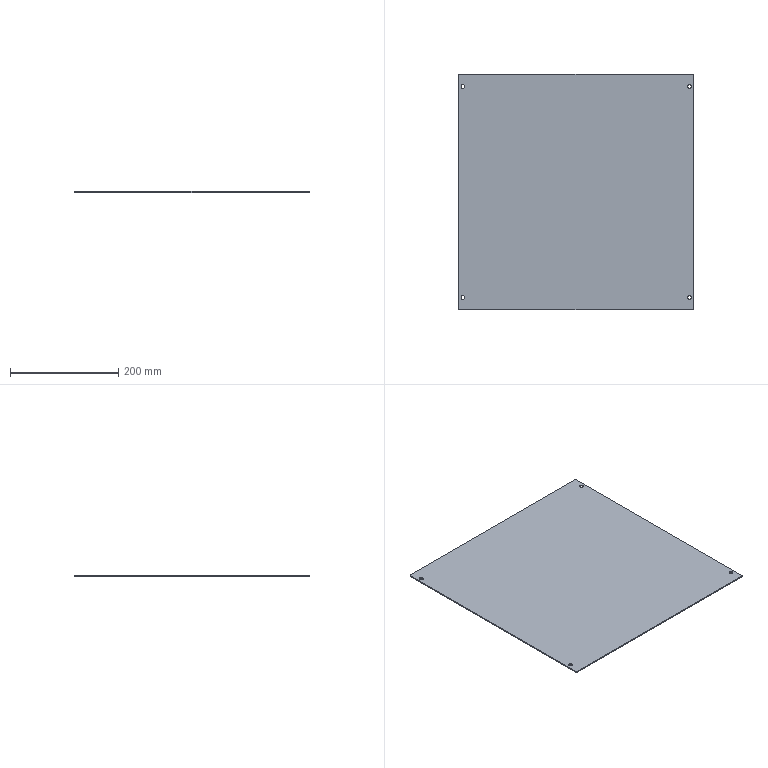Part | STEP file | Control Box Rear Closing Plate | 1 solid | 18 faces | box 433 x 435 x 2 mm | volume 376395 mm3 | cylinder 12 | plane 6 | commonest cylinder face diameters 7 x8 4 x4
STEP:
#1=CARTESIAN_POINT('',(-411.682,-25.867,-2.));
#2=VERTEX_POINT('',#1);
#3=CARTESIAN_POINT('',(-418.682,-25.867,-2.));
#4=VERTEX_POINT('',#3);
#5=CARTESIAN_POINT('',(-415.182,-25.867,-2.));
#6=DIRECTION('',(0.,0.,-1.));
#7=DIRECTION('',(1.,0.,0.));
#8=AXIS2_PLACEMENT_3D('',#5,#6,#7);
#9=CIRCLE('',#8,3.5);
#10=EDGE_CURVE('',#2,#4,#9,.T.);
#11=ORIENTED_EDGE('',*,*,#10,.T.);
#12=CARTESIAN_POINT('',(-418.682,-25.867,0.));
#13=VERTEX_POINT('',#12);
#14=CARTESIAN_POINT('',(-418.682,-25.867,-10.));
#15=DIRECTION('',(0.,0.,1.));
#16=VECTOR('',#15,1000.);
#17=LINE('',#14,#16);
#18=EDGE_CURVE('',#4,#13,#17,.T.);
#19=ORIENTED_EDGE('',*,*,#18,.T.);
#20=CARTESIAN_POINT('',(-411.682,-25.867,0.));
#21=VERTEX_POINT('',#20);
#22=CARTESIAN_POINT('',(-415.182,-25.867,0.));
#23=DIRECTION('',(0.,0.,-1.));
#24=DIRECTION('',(1.,0.,0.));
#25=AXIS2_PLACEMENT_3D('',#22,#23,#24);
#26=CIRCLE('',#25,3.5);
#27=EDGE_CURVE('',#21,#13,#26,.T.);
#28=ORIENTED_EDGE('',*,*,#27,.F.);
#29=CARTESIAN_POINT('',(-411.682,-25.867,-10.));
#30=DIRECTION('',(0.,0.,1.));
#31=VECTOR('',#30,1000.);
#32=LINE('',#29,#31);
#33=EDGE_CURVE('',#2,#21,#32,.T.);
#34=ORIENTED_EDGE('',*,*,#33,.F.);
#35=EDGE_LOOP('',(#11,#19,#28,#34));
#36=FACE_OUTER_BOUND('',#35,.T.);
#37=CARTESIAN_POINT('',(-415.182,-25.867,-10.));
#38=DIRECTION('',(0.,0.,1.));
#39=DIRECTION('',(1.,0.,0.));
#40=AXIS2_PLACEMENT_3D('',#37,#38,#39);
#41=CYLINDRICAL_SURFACE('',#40,3.5);
#42=ADVANCED_FACE('',(#36),#41,.F.);
#43=CARTESIAN_POINT('',(6.197,-25.867,-2.));
#44=VERTEX_POINT('',#43);
#45=CARTESIAN_POINT('',(-0.8031,-25.867,-2.));
#46=VERTEX_POINT('',#45);
#47=CARTESIAN_POINT('',(2.697,-25.867,-2.));
#48=DIRECTION('',(0.,0.,-1.));
#49=DIRECTION('',(1.,0.,0.));
#50=AXIS2_PLACEMENT_3D('',#47,#48,#49);
#51=CIRCLE('',#50,3.5);
#52=EDGE_CURVE('',#44,#46,#51,.T.);
#53=ORIENTED_EDGE('',*,*,#52,.T.);
#54=CARTESIAN_POINT('',(-0.8031,-25.867,0.));
#55=VERTEX_POINT('',#54);
#56=CARTESIAN_POINT('',(-0.8031,-25.867,-10.));
#57=DIRECTION('',(0.,0.,1.));
#58=VECTOR('',#57,1000.);
#59=LINE('',#56,#58);
#60=EDGE_CURVE('',#46,#55,#59,.T.);
#61=ORIENTED_EDGE('',*,*,#60,.T.);
#62=CARTESIAN_POINT('',(6.197,-25.867,0.));
#63=VERTEX_POINT('',#62);
#64=CARTESIAN_POINT('',(2.697,-25.867,0.));
#65=DIRECTION('',(0.,0.,-1.));
#66=DIRECTION('',(1.,0.,0.));
#67=AXIS2_PLACEMENT_3D('',#64,#65,#66);
#68=CIRCLE('',#67,3.5);
#69=EDGE_CURVE('',#63,#55,#68,.T.);
#70=ORIENTED_EDGE('',*,*,#69,.F.);
#71=CARTESIAN_POINT('',(6.197,-25.867,-10.));
#72=DIRECTION('',(0.,0.,1.));
#73=VECTOR('',#72,1000.);
#74=LINE('',#71,#73);
#75=EDGE_CURVE('',#44,#63,#74,.T.);
#76=ORIENTED_EDGE('',*,*,#75,.F.);
#77=EDGE_LOOP('',(#53,#61,#70,#76));
#78=FACE_OUTER_BOUND('',#77,.T.);
#79=CARTESIAN_POINT('',(2.697,-25.867,-10.));
#80=DIRECTION('',(0.,0.,1.));
#81=DIRECTION('',(1.,0.,0.));
#82=AXIS2_PLACEMENT_3D('',#79,#80,#81);
#83=CYLINDRICAL_SURFACE('',#82,3.5);
#84=ADVANCED_FACE('',(#78),#83,.F.);
#85=CARTESIAN_POINT('',(6.197,-414.867,-2.));
#86=VERTEX_POINT('',#85);
#87=CARTESIAN_POINT('',(-0.8031,-414.867,-2.));
#88=VERTEX_POINT('',#87);
#89=CARTESIAN_POINT('',(2.697,-414.867,-2.));
#90=DIRECTION('',(0.,0.,-1.));
#91=DIRECTION('',(1.,0.,0.));
#92=AXIS2_PLACEMENT_3D('',#89,#90,#91);
#93=CIRCLE('',#92,3.5);
#94=EDGE_CURVE('',#86,#88,#93,.T.);
#95=ORIENTED_EDGE('',*,*,#94,.T.);
#96=CARTESIAN_POINT('',(-0.8031,-414.867,0.));
#97=VERTEX_POINT('',#96);
#98=CARTESIAN_POINT('',(-0.8031,-414.867,-10.));
#99=DIRECTION('',(0.,0.,1.));
#100=VECTOR('',#99,1000.);
#101=LINE('',#98,#100);
#102=EDGE_CURVE('',#88,#97,#101,.T.);
#103=ORIENTED_EDGE('',*,*,#102,.T.);
#104=CARTESIAN_POINT('',(6.197,-414.867,0.));
#105=VERTEX_POINT('',#104);
#106=CARTESIAN_POINT('',(2.697,-414.867,0.));
#107=DIRECTION('',(0.,0.,-1.));
#108=DIRECTION('',(1.,0.,0.));
#109=AXIS2_PLACEMENT_3D('',#106,#107,#108);
#110=CIRCLE('',#109,3.5);
#111=EDGE_CURVE('',#105,#97,#110,.T.);
#112=ORIENTED_EDGE('',*,*,#111,.F.);
#113=CARTESIAN_POINT('',(6.197,-414.867,-10.));
#114=DIRECTION('',(0.,0.,1.));
#115=VECTOR('',#114,1000.);
#116=LINE('',#113,#115);
#117=EDGE_CURVE('',#86,#105,#116,.T.);
#118=ORIENTED_EDGE('',*,*,#117,.F.);
#119=EDGE_LOOP('',(#95,#103,#112,#118));
#120=FACE_OUTER_BOUND('',#119,.T.);
#121=CARTESIAN_POINT('',(2.697,-414.867,-10.));
#122=DIRECTION('',(0.,0.,1.));
#123=DIRECTION('',(1.,0.,0.));
#124=AXIS2_PLACEMENT_3D('',#121,#122,#123);
#125=CYLINDRICAL_SURFACE('',#124,3.5);
#126=ADVANCED_FACE('',(#120),#125,.F.);
#127=CARTESIAN_POINT('',(-411.682,-414.867,-2.));
#128=VERTEX_POINT('',#127);
#129=CARTESIAN_POINT('',(-418.682,-414.867,-2.));
#130=VERTEX_POINT('',#129);
#131=CARTESIAN_POINT('',(-415.182,-414.867,-2.));
#132=DIRECTION('',(0.,0.,-1.));
#133=DIRECTION('',(1.,0.,0.));
#134=AXIS2_PLACEMENT_3D('',#131,#132,#133);
#135=CIRCLE('',#134,3.5);
#136=EDGE_CURVE('',#128,#130,#135,.T.);
#137=ORIENTED_EDGE('',*,*,#136,.T.);
#138=CARTESIAN_POINT('',(-418.682,-414.867,0.));
#139=VERTEX_POINT('',#138);
#140=CARTESIAN_POINT('',(-418.682,-414.867,-10.));
#141=DIRECTION('',(0.,0.,1.));
#142=VECTOR('',#141,1000.);
#143=LINE('',#140,#142);
#144=EDGE_CURVE('',#130,#139,#143,.T.);
#145=ORIENTED_EDGE('',*,*,#144,.T.);
#146=CARTESIAN_POINT('',(-411.682,-414.867,0.));
#147=VERTEX_POINT('',#146);
#148=CARTESIAN_POINT('',(-415.182,-414.867,0.));
#149=DIRECTION('',(0.,0.,-1.));
#150=DIRECTION('',(1.,0.,0.));
#151=AXIS2_PLACEMENT_3D('',#148,#149,#150);
#152=CIRCLE('',#151,3.5);
#153=EDGE_CURVE('',#147,#139,#152,.T.);
#154=ORIENTED_EDGE('',*,*,#153,.F.);
#155=CARTESIAN_POINT('',(-411.682,-414.867,-10.));
#156=DIRECTION('',(0.,0.,1.));
#157=VECTOR('',#156,1000.);
#158=LINE('',#155,#157);
#159=EDGE_CURVE('',#128,#147,#158,.T.);
#160=ORIENTED_EDGE('',*,*,#159,.F.);
#161=EDGE_LOOP('',(#137,#145,#154,#160));
#162=FACE_OUTER_BOUND('',#161,.T.);
#163=CARTESIAN_POINT('',(-415.182,-414.867,-10.));
#164=DIRECTION('',(0.,0.,1.));
#165=DIRECTION('',(1.,0.,0.));
#166=AXIS2_PLACEMENT_3D('',#163,#164,#165);
#167=CYLINDRICAL_SURFACE('',#166,3.5);
#168=ADVANCED_FACE('',(#162),#167,.F.);
#169=CARTESIAN_POINT('',(7.818,-437.867,-2.));
#170=VERTEX_POINT('',#169);
#171=CARTESIAN_POINT('',(9.818,-435.867,-2.));
#172=VERTEX_POINT('',#171);
#173=CARTESIAN_POINT('',(7.818,-435.867,-2.));
#174=DIRECTION('',(0.,0.,1.));
#175=DIRECTION('',(1.,0.,0.));
#176=AXIS2_PLACEMENT_3D('',#173,#174,#175);
#177=CIRCLE('',#176,2.);
#178=EDGE_CURVE('',#170,#172,#177,.T.);
#179=ORIENTED_EDGE('',*,*,#178,.F.);
#180=CARTESIAN_POINT('',(-421.182,-437.867,-2.));
#181=VERTEX_POINT('',#180);
#182=CARTESIAN_POINT('',(0.,-437.867,-2.));
#183=DIRECTION('',(1.,0.,0.));
#184=VECTOR('',#183,1000.);
#185=LINE('',#182,#184);
#186=EDGE_CURVE('',#181,#170,#185,.T.);
#187=ORIENTED_EDGE('',*,*,#186,.F.);
#188=CARTESIAN_POINT('',(-423.182,-435.867,-2.));
#189=VERTEX_POINT('',#188);
#190=CARTESIAN_POINT('',(-421.182,-435.867,-2.));
#191=DIRECTION('',(0.,0.,1.));
#192=DIRECTION('',(1.,0.,0.));
#193=AXIS2_PLACEMENT_3D('',#190,#191,#192);
#194=CIRCLE('',#193,2.);
#195=EDGE_CURVE('',#189,#181,#194,.T.);
#196=ORIENTED_EDGE('',*,*,#195,.F.);
#197=CARTESIAN_POINT('',(-423.182,-4.867,-2.));
#198=VERTEX_POINT('',#197);
#199=CARTESIAN_POINT('',(-423.182,0.,-2.));
#200=DIRECTION('',(0.,-1.,0.));
#201=VECTOR('',#200,1000.);
#202=LINE('',#199,#201);
#203=EDGE_CURVE('',#198,#189,#202,.T.);
#204=ORIENTED_EDGE('',*,*,#203,.F.);
#205=CARTESIAN_POINT('',(-421.182,-2.867,-2.));
#206=VERTEX_POINT('',#205);
#207=CARTESIAN_POINT('',(-421.182,-4.867,-2.));
#208=DIRECTION('',(0.,0.,1.));
#209=DIRECTION('',(1.,0.,0.));
#210=AXIS2_PLACEMENT_3D('',#207,#208,#209);
#211=CIRCLE('',#210,2.);
#212=EDGE_CURVE('',#206,#198,#211,.T.);
#213=ORIENTED_EDGE('',*,*,#212,.F.);
#214=CARTESIAN_POINT('',(7.818,-2.867,-2.));
#215=VERTEX_POINT('',#214);
#216=CARTESIAN_POINT('',(0.,-2.867,-2.));
#217=DIRECTION('',(-1.,0.,0.));
#218=VECTOR('',#217,1000.);
#219=LINE('',#216,#218);
#220=EDGE_CURVE('',#215,#206,#219,.T.);
#221=ORIENTED_EDGE('',*,*,#220,.F.);
#222=CARTESIAN_POINT('',(9.818,-4.867,-2.));
#223=VERTEX_POINT('',#222);
#224=CARTESIAN_POINT('',(7.818,-4.867,-2.));
#225=DIRECTION('',(0.,0.,1.));
#226=DIRECTION('',(1.,0.,0.));
#227=AXIS2_PLACEMENT_3D('',#224,#225,#226);
#228=CIRCLE('',#227,2.);
#229=EDGE_CURVE('',#223,#215,#228,.T.);
#230=ORIENTED_EDGE('',*,*,#229,.F.);
#231=CARTESIAN_POINT('',(9.818,0.,-2.));
#232=DIRECTION('',(0.,1.,0.));
#233=VECTOR('',#232,1000.);
#234=LINE('',#231,#233);
#235=EDGE_CURVE('',#172,#223,#234,.T.);
#236=ORIENTED_EDGE('',*,*,#235,.F.);
#237=EDGE_LOOP('',(#179,#187,#196,#204,#213,#221,#230,#236));
#238=FACE_OUTER_BOUND('',#237,.T.);
#239=ORIENTED_EDGE('',*,*,#10,.F.);
#240=CARTESIAN_POINT('',(-415.182,-25.867,-2.));
#241=DIRECTION('',(0.,0.,-1.));
#242=DIRECTION('',(1.,0.,0.));
#243=AXIS2_PLACEMENT_3D('',#240,#241,#242);
#244=CIRCLE('',#243,3.5);
#245=EDGE_CURVE('',#4,#2,#244,.T.);
#246=ORIENTED_EDGE('',*,*,#245,.F.);
#247=EDGE_LOOP('',(#239,#246));
#248=FACE_BOUND('',#247,.T.);
#249=ORIENTED_EDGE('',*,*,#52,.F.);
#250=CARTESIAN_POINT('',(2.697,-25.867,-2.));
#251=DIRECTION('',(0.,0.,-1.));
#252=DIRECTION('',(1.,0.,0.));
#253=AXIS2_PLACEMENT_3D('',#250,#251,#252);
#254=CIRCLE('',#253,3.5);
#255=EDGE_CURVE('',#46,#44,#254,.T.);
#256=ORIENTED_EDGE('',*,*,#255,.F.);
#257=EDGE_LOOP('',(#249,#256));
#258=FACE_BOUND('',#257,.T.);
#259=ORIENTED_EDGE('',*,*,#94,.F.);
#260=CARTESIAN_POINT('',(2.697,-414.867,-2.));
#261=DIRECTION('',(0.,0.,-1.));
#262=DIRECTION('',(1.,0.,0.));
#263=AXIS2_PLACEMENT_3D('',#260,#261,#262);
#264=CIRCLE('',#263,3.5);
#265=EDGE_CURVE('',#88,#86,#264,.T.);
#266=ORIENTED_EDGE('',*,*,#265,.F.);
#267=EDGE_LOOP('',(#259,#266));
#268=FACE_BOUND('',#267,.T.);
#269=ORIENTED_EDGE('',*,*,#136,.F.);
#270=CARTESIAN_POINT('',(-415.182,-414.867,-2.));
#271=DIRECTION('',(0.,0.,-1.));
#272=DIRECTION('',(1.,0.,0.));
#273=AXIS2_PLACEMENT_3D('',#270,#271,#272);
#274=CIRCLE('',#273,3.5);
#275=EDGE_CURVE('',#130,#128,#274,.T.);
#276=ORIENTED_EDGE('',*,*,#275,.F.);
#277=EDGE_LOOP('',(#269,#276));
#278=FACE_BOUND('',#277,.T.);
#279=CARTESIAN_POINT('',(0.,0.,-2.));
#280=DIRECTION('',(0.,0.,1.));
#281=DIRECTION('',(1.,0.,0.));
#282=AXIS2_PLACEMENT_3D('',#279,#280,#281);
#283=PLANE('',#282);
#284=ADVANCED_FACE('',(#238,#248,#258,#268,#278),#283,.F.);
#285=ORIENTED_EDGE('',*,*,#235,.T.);
#286=CARTESIAN_POINT('',(9.818,-4.867,0.));
#287=VERTEX_POINT('',#286);
#288=CARTESIAN_POINT('',(9.818,-4.867,-2.));
#289=DIRECTION('',(0.,0.,1.));
#290=VECTOR('',#289,1000.);
#291=LINE('',#288,#290);
#292=EDGE_CURVE('',#223,#287,#291,.T.);
#293=ORIENTED_EDGE('',*,*,#292,.T.);
#294=CARTESIAN_POINT('',(9.818,-435.867,0.));
#295=VERTEX_POINT('',#294);
#296=CARTESIAN_POINT('',(9.818,-2.867,0.));
#297=DIRECTION('',(0.,-1.,0.));
#298=VECTOR('',#297,1000.);
#299=LINE('',#296,#298);
#300=EDGE_CURVE('',#287,#295,#299,.T.);
#301=ORIENTED_EDGE('',*,*,#300,.T.);
#302=CARTESIAN_POINT('',(9.818,-435.867,-2.));
#303=DIRECTION('',(0.,0.,-1.));
#304=VECTOR('',#303,1000.);
#305=LINE('',#302,#304);
#306=EDGE_CURVE('',#295,#172,#305,.T.);
#307=ORIENTED_EDGE('',*,*,#306,.T.);
#308=EDGE_LOOP('',(#285,#293,#301,#307));
#309=FACE_OUTER_BOUND('',#308,.T.);
#310=CARTESIAN_POINT('',(9.818,-2.867,-2.));
#311=DIRECTION('',(1.,0.,0.));
#312=DIRECTION('',(0.,1.,0.));
#313=AXIS2_PLACEMENT_3D('',#310,#311,#312);
#314=PLANE('',#313);
#315=ADVANCED_FACE('',(#309),#314,.T.);
#316=CARTESIAN_POINT('',(7.818,-437.867,0.));
#317=VERTEX_POINT('',#316);
#318=CARTESIAN_POINT('',(7.818,-435.867,0.));
#319=DIRECTION('',(0.,0.,-1.));
#320=DIRECTION('',(1.,0.,0.));
#321=AXIS2_PLACEMENT_3D('',#318,#319,#320);
#322=CIRCLE('',#321,2.);
#323=EDGE_CURVE('',#295,#317,#322,.T.);
#324=ORIENTED_EDGE('',*,*,#323,.T.);
#325=CARTESIAN_POINT('',(7.818,-437.867,-2.));
#326=DIRECTION('',(0.,0.,-1.));
#327=VECTOR('',#326,1000.);
#328=LINE('',#325,#327);
#329=EDGE_CURVE('',#317,#170,#328,.T.);
#330=ORIENTED_EDGE('',*,*,#329,.T.);
#331=ORIENTED_EDGE('',*,*,#178,.T.);
#332=ORIENTED_EDGE('',*,*,#306,.F.);
#333=EDGE_LOOP('',(#324,#330,#331,#332));
#334=FACE_OUTER_BOUND('',#333,.T.);
#335=CARTESIAN_POINT('',(7.818,-435.867,-2.));
#336=DIRECTION('',(0.,0.,1.));
#337=DIRECTION('',(1.,0.,0.));
#338=AXIS2_PLACEMENT_3D('',#335,#336,#337);
#339=CYLINDRICAL_SURFACE('',#338,2.);
#340=ADVANCED_FACE('',(#334),#339,.T.);
#341=CARTESIAN_POINT('',(-421.182,-437.867,0.));
#342=VERTEX_POINT('',#341);
#343=CARTESIAN_POINT('',(-423.182,-437.867,0.));
#344=DIRECTION('',(-1.,0.,0.));
#345=VECTOR('',#344,1000.);
#346=LINE('',#343,#345);
#347=EDGE_CURVE('',#317,#342,#346,.T.);
#348=ORIENTED_EDGE('',*,*,#347,.T.);
#349=CARTESIAN_POINT('',(-421.182,-437.867,-2.));
#350=DIRECTION('',(0.,0.,-1.));
#351=VECTOR('',#350,1000.);
#352=LINE('',#349,#351);
#353=EDGE_CURVE('',#342,#181,#352,.T.);
#354=ORIENTED_EDGE('',*,*,#353,.T.);
#355=ORIENTED_EDGE('',*,*,#186,.T.);
#356=ORIENTED_EDGE('',*,*,#329,.F.);
#357=EDGE_LOOP('',(#348,#354,#355,#356));
#358=FACE_OUTER_BOUND('',#357,.T.);
#359=CARTESIAN_POINT('',(-423.182,-437.867,-2.));
#360=DIRECTION('',(0.,-1.,0.));
#361=DIRECTION('',(0.,0.,-1.));
#362=AXIS2_PLACEMENT_3D('',#359,#360,#361);
#363=PLANE('',#362);
#364=ADVANCED_FACE('',(#358),#363,.T.);
#365=CARTESIAN_POINT('',(-423.182,-435.867,0.));
#366=VERTEX_POINT('',#365);
#367=CARTESIAN_POINT('',(-421.182,-435.867,0.));
#368=DIRECTION('',(0.,0.,-1.));
#369=DIRECTION('',(1.,0.,0.));
#370=AXIS2_PLACEMENT_3D('',#367,#368,#369);
#371=CIRCLE('',#370,2.);
#372=EDGE_CURVE('',#342,#366,#371,.T.);
#373=ORIENTED_EDGE('',*,*,#372,.T.);
#374=CARTESIAN_POINT('',(-423.182,-435.867,-2.));
#375=DIRECTION('',(0.,0.,-1.));
#376=VECTOR('',#375,1000.);
#377=LINE('',#374,#376);
#378=EDGE_CURVE('',#366,#189,#377,.T.);
#379=ORIENTED_EDGE('',*,*,#378,.T.);
#380=ORIENTED_EDGE('',*,*,#195,.T.);
#381=ORIENTED_EDGE('',*,*,#353,.F.);
#382=EDGE_LOOP('',(#373,#379,#380,#381));
#383=FACE_OUTER_BOUND('',#382,.T.);
#384=CARTESIAN_POINT('',(-421.182,-435.867,-2.));
#385=DIRECTION('',(0.,0.,1.));
#386=DIRECTION('',(1.,0.,0.));
#387=AXIS2_PLACEMENT_3D('',#384,#385,#386);
#388=CYLINDRICAL_SURFACE('',#387,2.);
#389=ADVANCED_FACE('',(#383),#388,.T.);
#390=CARTESIAN_POINT('',(-423.182,-4.867,0.));
#391=VERTEX_POINT('',#390);
#392=CARTESIAN_POINT('',(-423.182,-2.867,0.));
#393=DIRECTION('',(0.,1.,0.));
#394=VECTOR('',#393,1000.);
#395=LINE('',#392,#394);
#396=EDGE_CURVE('',#366,#391,#395,.T.);
#397=ORIENTED_EDGE('',*,*,#396,.T.);
#398=CARTESIAN_POINT('',(-423.182,-4.867,-2.));
#399=DIRECTION('',(0.,0.,-1.));
#400=VECTOR('',#399,1000.);
#401=LINE('',#398,#400);
#402=EDGE_CURVE('',#391,#198,#401,.T.);
#403=ORIENTED_EDGE('',*,*,#402,.T.);
#404=ORIENTED_EDGE('',*,*,#203,.T.);
#405=ORIENTED_EDGE('',*,*,#378,.F.);
#406=EDGE_LOOP('',(#397,#403,#404,#405));
#407=FACE_OUTER_BOUND('',#406,.T.);
#408=CARTESIAN_POINT('',(-423.182,-2.867,-2.));
#409=DIRECTION('',(-1.,0.,0.));
#410=DIRECTION('',(0.,0.,1.));
#411=AXIS2_PLACEMENT_3D('',#408,#409,#410);
#412=PLANE('',#411);
#413=ADVANCED_FACE('',(#407),#412,.T.);
#414=CARTESIAN_POINT('',(-421.182,-2.867,0.));
#415=VERTEX_POINT('',#414);
#416=CARTESIAN_POINT('',(-421.182,-4.867,0.));
#417=DIRECTION('',(0.,0.,-1.));
#418=DIRECTION('',(1.,0.,0.));
#419=AXIS2_PLACEMENT_3D('',#416,#417,#418);
#420=CIRCLE('',#419,2.);
#421=EDGE_CURVE('',#391,#415,#420,.T.);
#422=ORIENTED_EDGE('',*,*,#421,.T.);
#423=CARTESIAN_POINT('',(-421.182,-2.867,-2.));
#424=DIRECTION('',(0.,0.,-1.));
#425=VECTOR('',#424,1000.);
#426=LINE('',#423,#425);
#427=EDGE_CURVE('',#415,#206,#426,.T.);
#428=ORIENTED_EDGE('',*,*,#427,.T.);
#429=ORIENTED_EDGE('',*,*,#212,.T.);
#430=ORIENTED_EDGE('',*,*,#402,.F.);
#431=EDGE_LOOP('',(#422,#428,#429,#430));
#432=FACE_OUTER_BOUND('',#431,.T.);
#433=CARTESIAN_POINT('',(-421.182,-4.867,-2.));
#434=DIRECTION('',(0.,0.,1.));
#435=DIRECTION('',(1.,0.,0.));
#436=AXIS2_PLACEMENT_3D('',#433,#434,#435);
#437=CYLINDRICAL_SURFACE('',#436,2.);
#438=ADVANCED_FACE('',(#432),#437,.T.);
#439=CARTESIAN_POINT('',(7.818,-2.867,0.));
#440=VERTEX_POINT('',#439);
#441=CARTESIAN_POINT('',(-423.182,-2.867,0.));
#442=DIRECTION('',(1.,0.,0.));
#443=VECTOR('',#442,1000.);
#444=LINE('',#441,#443);
#445=EDGE_CURVE('',#415,#440,#444,.T.);
#446=ORIENTED_EDGE('',*,*,#445,.T.);
#447=CARTESIAN_POINT('',(7.818,-2.867,-2.));
#448=DIRECTION('',(0.,0.,-1.));
#449=VECTOR('',#448,1000.);
#450=LINE('',#447,#449);
#451=EDGE_CURVE('',#440,#215,#450,.T.);
#452=ORIENTED_EDGE('',*,*,#451,.T.);
#453=ORIENTED_EDGE('',*,*,#220,.T.);
#454=ORIENTED_EDGE('',*,*,#427,.F.);
#455=EDGE_LOOP('',(#446,#452,#453,#454));
#456=FACE_OUTER_BOUND('',#455,.T.);
#457=CARTESIAN_POINT('',(-423.182,-2.867,-2.));
#458=DIRECTION('',(0.,1.,0.));
#459=DIRECTION('',(0.,0.,1.));
#460=AXIS2_PLACEMENT_3D('',#457,#458,#459);
#461=PLANE('',#460);
#462=ADVANCED_FACE('',(#456),#461,.T.);
#463=CARTESIAN_POINT('',(7.818,-4.867,0.));
#464=DIRECTION('',(0.,0.,-1.));
#465=DIRECTION('',(1.,0.,0.));
#466=AXIS2_PLACEMENT_3D('',#463,#464,#465);
#467=CIRCLE('',#466,2.);
#468=EDGE_CURVE('',#440,#287,#467,.T.);
#469=ORIENTED_EDGE('',*,*,#468,.T.);
#470=ORIENTED_EDGE('',*,*,#292,.F.);
#471=ORIENTED_EDGE('',*,*,#229,.T.);
#472=ORIENTED_EDGE('',*,*,#451,.F.);
#473=EDGE_LOOP('',(#469,#470,#471,#472));
#474=FACE_OUTER_BOUND('',#473,.T.);
#475=CARTESIAN_POINT('',(7.818,-4.867,-2.));
#476=DIRECTION('',(0.,0.,1.));
#477=DIRECTION('',(1.,0.,0.));
#478=AXIS2_PLACEMENT_3D('',#475,#476,#477);
#479=CYLINDRICAL_SURFACE('',#478,2.);
#480=ADVANCED_FACE('',(#474),#479,.T.);
#481=ORIENTED_EDGE('',*,*,#18,.F.);
#482=ORIENTED_EDGE('',*,*,#245,.T.);
#483=ORIENTED_EDGE('',*,*,#33,.T.);
#484=CARTESIAN_POINT('',(-415.182,-25.867,0.));
#485=DIRECTION('',(0.,0.,-1.));
#486=DIRECTION('',(1.,0.,0.));
#487=AXIS2_PLACEMENT_3D('',#484,#485,#486);
#488=CIRCLE('',#487,3.5);
#489=EDGE_CURVE('',#13,#21,#488,.T.);
#490=ORIENTED_EDGE('',*,*,#489,.F.);
#491=EDGE_LOOP('',(#481,#482,#483,#490));
#492=FACE_OUTER_BOUND('',#491,.T.);
#493=CARTESIAN_POINT('',(-415.182,-25.867,-10.));
#494=DIRECTION('',(0.,0.,1.));
#495=DIRECTION('',(1.,0.,0.));
#496=AXIS2_PLACEMENT_3D('',#493,#494,#495);
#497=CYLINDRICAL_SURFACE('',#496,3.5);
#498=ADVANCED_FACE('',(#492),#497,.F.);
#499=ORIENTED_EDGE('',*,*,#60,.F.);
#500=ORIENTED_EDGE('',*,*,#255,.T.);
#501=ORIENTED_EDGE('',*,*,#75,.T.);
#502=CARTESIAN_POINT('',(2.697,-25.867,0.));
#503=DIRECTION('',(0.,0.,-1.));
#504=DIRECTION('',(1.,0.,0.));
#505=AXIS2_PLACEMENT_3D('',#502,#503,#504);
#506=CIRCLE('',#505,3.5);
#507=EDGE_CURVE('',#55,#63,#506,.T.);
#508=ORIENTED_EDGE('',*,*,#507,.F.);
#509=EDGE_LOOP('',(#499,#500,#501,#508));
#510=FACE_OUTER_BOUND('',#509,.T.);
#511=CARTESIAN_POINT('',(2.697,-25.867,-10.));
#512=DIRECTION('',(0.,0.,1.));
#513=DIRECTION('',(1.,0.,0.));
#514=AXIS2_PLACEMENT_3D('',#511,#512,#513);
#515=CYLINDRICAL_SURFACE('',#514,3.5);
#516=ADVANCED_FACE('',(#510),#515,.F.);
#517=ORIENTED_EDGE('',*,*,#102,.F.);
#518=ORIENTED_EDGE('',*,*,#265,.T.);
#519=ORIENTED_EDGE('',*,*,#117,.T.);
#520=CARTESIAN_POINT('',(2.697,-414.867,0.));
#521=DIRECTION('',(0.,0.,-1.));
#522=DIRECTION('',(1.,0.,0.));
#523=AXIS2_PLACEMENT_3D('',#520,#521,#522);
#524=CIRCLE('',#523,3.5);
#525=EDGE_CURVE('',#97,#105,#524,.T.);
#526=ORIENTED_EDGE('',*,*,#525,.F.);
#527=EDGE_LOOP('',(#517,#518,#519,#526));
#528=FACE_OUTER_BOUND('',#527,.T.);
#529=CARTESIAN_POINT('',(2.697,-414.867,-10.));
#530=DIRECTION('',(0.,0.,1.));
#531=DIRECTION('',(1.,0.,0.));
#532=AXIS2_PLACEMENT_3D('',#529,#530,#531);
#533=CYLINDRICAL_SURFACE('',#532,3.5);
#534=ADVANCED_FACE('',(#528),#533,.F.);
#535=ORIENTED_EDGE('',*,*,#144,.F.);
#536=ORIENTED_EDGE('',*,*,#275,.T.);
#537=ORIENTED_EDGE('',*,*,#159,.T.);
#538=CARTESIAN_POINT('',(-415.182,-414.867,0.));
#539=DIRECTION('',(0.,0.,-1.));
#540=DIRECTION('',(1.,0.,0.));
#541=AXIS2_PLACEMENT_3D('',#538,#539,#540);
#542=CIRCLE('',#541,3.5);
#543=EDGE_CURVE('',#139,#147,#542,.T.);
#544=ORIENTED_EDGE('',*,*,#543,.F.);
#545=EDGE_LOOP('',(#535,#536,#537,#544));
#546=FACE_OUTER_BOUND('',#545,.T.);
#547=CARTESIAN_POINT('',(-415.182,-414.867,-10.));
#548=DIRECTION('',(0.,0.,1.));
#549=DIRECTION('',(1.,0.,0.));
#550=AXIS2_PLACEMENT_3D('',#547,#548,#549);
#551=CYLINDRICAL_SURFACE('',#550,3.5);
#552=ADVANCED_FACE('',(#546),#551,.F.);
#553=ORIENTED_EDGE('',*,*,#396,.F.);
#554=ORIENTED_EDGE('',*,*,#372,.F.);
#555=ORIENTED_EDGE('',*,*,#347,.F.);
#556=ORIENTED_EDGE('',*,*,#323,.F.);
#557=ORIENTED_EDGE('',*,*,#300,.F.);
#558=ORIENTED_EDGE('',*,*,#468,.F.);
#559=ORIENTED_EDGE('',*,*,#445,.F.);
#560=ORIENTED_EDGE('',*,*,#421,.F.);
#561=EDGE_LOOP('',(#553,#554,#555,#556,#557,#558,#559,#560));
#562=FACE_OUTER_BOUND('',#561,.T.);
#563=ORIENTED_EDGE('',*,*,#27,.T.);
#564=ORIENTED_EDGE('',*,*,#489,.T.);
#565=EDGE_LOOP('',(#563,#564));
#566=FACE_BOUND('',#565,.T.);
#567=ORIENTED_EDGE('',*,*,#69,.T.);
#568=ORIENTED_EDGE('',*,*,#507,.T.);
#569=EDGE_LOOP('',(#567,#568));
#570=FACE_BOUND('',#569,.T.);
#571=ORIENTED_EDGE('',*,*,#111,.T.);
#572=ORIENTED_EDGE('',*,*,#525,.T.);
#573=EDGE_LOOP('',(#571,#572));
#574=FACE_BOUND('',#573,.T.);
#575=ORIENTED_EDGE('',*,*,#153,.T.);
#576=ORIENTED_EDGE('',*,*,#543,.T.);
#577=EDGE_LOOP('',(#575,#576));
#578=FACE_BOUND('',#577,.T.);
#579=CARTESIAN_POINT('',(0.,0.,0.));
#580=DIRECTION('',(0.,0.,1.));
#581=DIRECTION('',(1.,0.,0.));
#582=AXIS2_PLACEMENT_3D('',#579,#580,#581);
#583=PLANE('',#582);
#584=ADVANCED_FACE('',(#562,#566,#570,#574,#578),#583,.T.);
#585=CLOSED_SHELL('',(#42,#84,#126,#168,#284,#315,#340,#364,#389,#413,#438,#462,#480,#498,#516,#534,#552,#584));
#586=MANIFOLD_SOLID_BREP('',#585);
#587=CARTESIAN_POINT('',(0.,0.,0.));
#588=DIRECTION('',(0.,0.,1.));
#589=DIRECTION('',(1.,0.,0.));
#590=AXIS2_PLACEMENT_3D('',#587,#588,#589);
#591=(LENGTH_UNIT()NAMED_UNIT(*)SI_UNIT(.MILLI.,.METRE.));
#592=UNCERTAINTY_MEASURE_WITH_UNIT(LENGTH_MEASURE(0.00001),#591,'','');
#593=(NAMED_UNIT(*)PLANE_ANGLE_UNIT()SI_UNIT($,.RADIAN.));
#594=(NAMED_UNIT(*)SI_UNIT($,.STERADIAN.)SOLID_ANGLE_UNIT());
#595=(GEOMETRIC_REPRESENTATION_CONTEXT(3)GLOBAL_UNCERTAINTY_ASSIGNED_CONTEXT((#592))GLOBAL_UNIT_ASSIGNED_CONTEXT((#591,#593,#594))REPRESENTATION_CONTEXT('',''));
#596=ADVANCED_BREP_SHAPE_REPRESENTATION('',(#586,#590),#595);